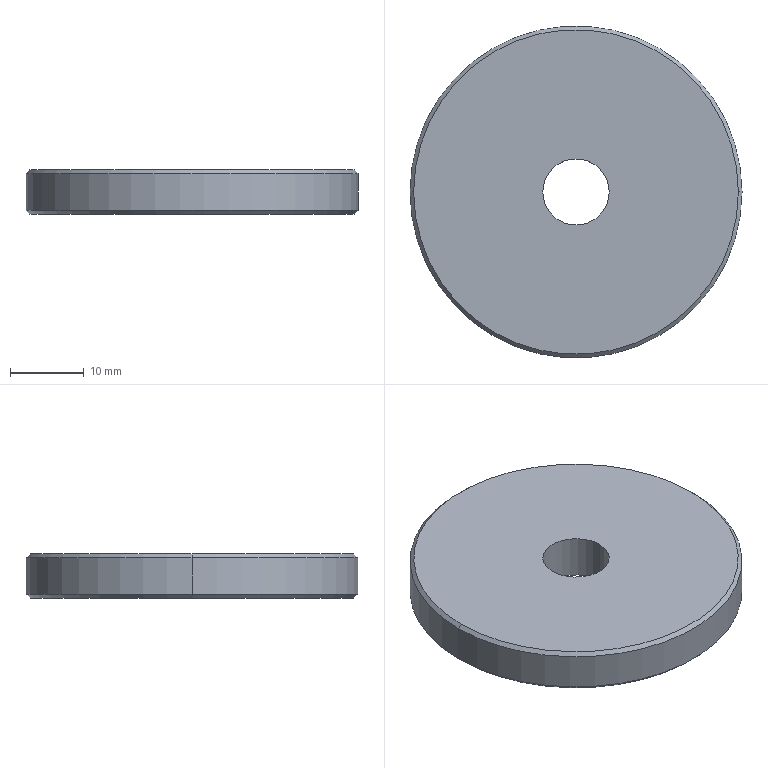Part | SolidWorks | features Chamfer 1, Extrusion 1 | 1 solid | 10 faces | box 45 x 45 x 6 mm | volume 9126 mm3 | cone 4 | cylinder 4 | plane 2 | commonest cylinder face diameters 9 x2 45 x2
STEP:
#1=CARTESIAN_POINT('',(22.,0.,6.));
#2=VERTEX_POINT('',#1);
#3=CARTESIAN_POINT('',(-22.,0.,6.));
#4=VERTEX_POINT('',#3);
#5=CARTESIAN_POINT('',(0.,0.,6.));
#6=DIRECTION('',(0.,0.,1.));
#7=DIRECTION('',(1.,0.,0.));
#8=AXIS2_PLACEMENT_3D('',#5,#6,#7);
#9=CIRCLE('',#8,22.);
#10=EDGE_CURVE('',#2,#4,#9,.T.);
#11=ORIENTED_EDGE('',*,*,#10,.F.);
#12=CARTESIAN_POINT('',(22.5,0.,5.5));
#13=VERTEX_POINT('',#12);
#14=CARTESIAN_POINT('',(22.,0.,6.));
#15=DIRECTION('',(0.7071,0.,-0.7071));
#16=VECTOR('',#15,1000.);
#17=LINE('',#14,#16);
#18=EDGE_CURVE('',#2,#13,#17,.T.);
#19=ORIENTED_EDGE('',*,*,#18,.T.);
#20=CARTESIAN_POINT('',(-22.5,0.,5.5));
#21=VERTEX_POINT('',#20);
#22=CARTESIAN_POINT('',(0.,0.,5.5));
#23=DIRECTION('',(0.,0.,-1.));
#24=DIRECTION('',(1.,0.,0.));
#25=AXIS2_PLACEMENT_3D('',#22,#23,#24);
#26=CIRCLE('',#25,22.5);
#27=EDGE_CURVE('',#21,#13,#26,.T.);
#28=ORIENTED_EDGE('',*,*,#27,.F.);
#29=CARTESIAN_POINT('',(-22.,0.,6.));
#30=DIRECTION('',(-0.7071,0.,-0.7071));
#31=VECTOR('',#30,1000.);
#32=LINE('',#29,#31);
#33=EDGE_CURVE('',#4,#21,#32,.T.);
#34=ORIENTED_EDGE('',*,*,#33,.F.);
#35=EDGE_LOOP('',(#11,#19,#28,#34));
#36=FACE_OUTER_BOUND('',#35,.T.);
#37=CARTESIAN_POINT('',(0.,0.,6.));
#38=DIRECTION('',(0.,0.,-1.));
#39=DIRECTION('',(-1.,0.,0.));
#40=AXIS2_PLACEMENT_3D('',#37,#38,#39);
#41=CONICAL_SURFACE('',#40,22.,0.7854);
#42=ADVANCED_FACE('',(#36),#41,.T.);
#43=CARTESIAN_POINT('',(-22.,0.,0.));
#44=VERTEX_POINT('',#43);
#45=CARTESIAN_POINT('',(22.,0.,0.));
#46=VERTEX_POINT('',#45);
#47=CARTESIAN_POINT('',(0.,0.,0.));
#48=DIRECTION('',(0.,0.,-1.));
#49=DIRECTION('',(1.,0.,0.));
#50=AXIS2_PLACEMENT_3D('',#47,#48,#49);
#51=CIRCLE('',#50,22.);
#52=EDGE_CURVE('',#44,#46,#51,.T.);
#53=ORIENTED_EDGE('',*,*,#52,.F.);
#54=CARTESIAN_POINT('',(-22.5,0.,0.5));
#55=VERTEX_POINT('',#54);
#56=CARTESIAN_POINT('',(-22.5,0.,0.5));
#57=DIRECTION('',(-0.7071,0.,0.7071));
#58=VECTOR('',#57,1000.);
#59=LINE('',#56,#58);
#60=EDGE_CURVE('',#44,#55,#59,.T.);
#61=ORIENTED_EDGE('',*,*,#60,.T.);
#62=CARTESIAN_POINT('',(22.5,0.,0.5));
#63=VERTEX_POINT('',#62);
#64=CARTESIAN_POINT('',(0.,0.,0.5));
#65=DIRECTION('',(0.,0.,1.));
#66=DIRECTION('',(1.,0.,0.));
#67=AXIS2_PLACEMENT_3D('',#64,#65,#66);
#68=CIRCLE('',#67,22.5);
#69=EDGE_CURVE('',#63,#55,#68,.T.);
#70=ORIENTED_EDGE('',*,*,#69,.F.);
#71=CARTESIAN_POINT('',(22.5,0.,0.5));
#72=DIRECTION('',(0.7071,0.,0.7071));
#73=VECTOR('',#72,1000.);
#74=LINE('',#71,#73);
#75=EDGE_CURVE('',#46,#63,#74,.T.);
#76=ORIENTED_EDGE('',*,*,#75,.F.);
#77=EDGE_LOOP('',(#53,#61,#70,#76));
#78=FACE_OUTER_BOUND('',#77,.T.);
#79=CARTESIAN_POINT('',(0.,0.,0.5));
#80=DIRECTION('',(0.,0.,1.));
#81=DIRECTION('',(1.,0.,0.));
#82=AXIS2_PLACEMENT_3D('',#79,#80,#81);
#83=CONICAL_SURFACE('',#82,22.5,0.7854);
#84=ADVANCED_FACE('',(#78),#83,.T.);
#85=CARTESIAN_POINT('',(-4.5,0.,6.));
#86=VERTEX_POINT('',#85);
#87=CARTESIAN_POINT('',(4.5,0.,6.));
#88=VERTEX_POINT('',#87);
#89=CARTESIAN_POINT('',(0.,0.,6.));
#90=DIRECTION('',(0.,0.,1.));
#91=DIRECTION('',(1.,0.,0.));
#92=AXIS2_PLACEMENT_3D('',#89,#90,#91);
#93=CIRCLE('',#92,4.5);
#94=EDGE_CURVE('',#86,#88,#93,.T.);
#95=ORIENTED_EDGE('',*,*,#94,.T.);
#96=CARTESIAN_POINT('',(4.5,0.,0.));
#97=VERTEX_POINT('',#96);
#98=CARTESIAN_POINT('',(4.5,0.,6.));
#99=DIRECTION('',(0.,0.,-1.));
#100=VECTOR('',#99,1000.);
#101=LINE('',#98,#100);
#102=EDGE_CURVE('',#88,#97,#101,.T.);
#103=ORIENTED_EDGE('',*,*,#102,.T.);
#104=CARTESIAN_POINT('',(-4.5,0.,0.));
#105=VERTEX_POINT('',#104);
#106=CARTESIAN_POINT('',(0.,0.,0.));
#107=DIRECTION('',(0.,0.,1.));
#108=DIRECTION('',(1.,0.,0.));
#109=AXIS2_PLACEMENT_3D('',#106,#107,#108);
#110=CIRCLE('',#109,4.5);
#111=EDGE_CURVE('',#105,#97,#110,.T.);
#112=ORIENTED_EDGE('',*,*,#111,.F.);
#113=CARTESIAN_POINT('',(-4.5,0.,6.));
#114=DIRECTION('',(0.,0.,-1.));
#115=VECTOR('',#114,1000.);
#116=LINE('',#113,#115);
#117=EDGE_CURVE('',#86,#105,#116,.T.);
#118=ORIENTED_EDGE('',*,*,#117,.F.);
#119=EDGE_LOOP('',(#95,#103,#112,#118));
#120=FACE_OUTER_BOUND('',#119,.T.);
#121=CARTESIAN_POINT('',(0.,0.,6.));
#122=DIRECTION('',(0.,0.,-1.));
#123=DIRECTION('',(-1.,0.,0.));
#124=AXIS2_PLACEMENT_3D('',#121,#122,#123);
#125=CYLINDRICAL_SURFACE('',#124,4.5);
#126=ADVANCED_FACE('',(#120),#125,.F.);
#127=ORIENTED_EDGE('',*,*,#27,.T.);
#128=CARTESIAN_POINT('',(22.5,0.,6.));
#129=DIRECTION('',(0.,0.,-1.));
#130=VECTOR('',#129,1000.);
#131=LINE('',#128,#130);
#132=EDGE_CURVE('',#13,#63,#131,.T.);
#133=ORIENTED_EDGE('',*,*,#132,.T.);
#134=ORIENTED_EDGE('',*,*,#69,.T.);
#135=CARTESIAN_POINT('',(-22.5,0.,6.));
#136=DIRECTION('',(0.,0.,-1.));
#137=VECTOR('',#136,1000.);
#138=LINE('',#135,#137);
#139=EDGE_CURVE('',#21,#55,#138,.T.);
#140=ORIENTED_EDGE('',*,*,#139,.F.);
#141=EDGE_LOOP('',(#127,#133,#134,#140));
#142=FACE_OUTER_BOUND('',#141,.T.);
#143=CARTESIAN_POINT('',(0.,0.,6.));
#144=DIRECTION('',(0.,0.,-1.));
#145=DIRECTION('',(-1.,0.,0.));
#146=AXIS2_PLACEMENT_3D('',#143,#144,#145);
#147=CYLINDRICAL_SURFACE('',#146,22.5);
#148=ADVANCED_FACE('',(#142),#147,.T.);
#149=CARTESIAN_POINT('',(0.,0.,6.));
#150=DIRECTION('',(0.,0.,1.));
#151=DIRECTION('',(1.,0.,0.));
#152=AXIS2_PLACEMENT_3D('',#149,#150,#151);
#153=CIRCLE('',#152,22.);
#154=EDGE_CURVE('',#4,#2,#153,.T.);
#155=ORIENTED_EDGE('',*,*,#154,.T.);
#156=ORIENTED_EDGE('',*,*,#10,.T.);
#157=EDGE_LOOP('',(#155,#156));
#158=FACE_OUTER_BOUND('',#157,.T.);
#159=ORIENTED_EDGE('',*,*,#94,.F.);
#160=CARTESIAN_POINT('',(0.,0.,6.));
#161=DIRECTION('',(0.,0.,1.));
#162=DIRECTION('',(1.,0.,0.));
#163=AXIS2_PLACEMENT_3D('',#160,#161,#162);
#164=CIRCLE('',#163,4.5);
#165=EDGE_CURVE('',#88,#86,#164,.T.);
#166=ORIENTED_EDGE('',*,*,#165,.F.);
#167=EDGE_LOOP('',(#159,#166));
#168=FACE_BOUND('',#167,.T.);
#169=CARTESIAN_POINT('',(0.,0.,6.));
#170=DIRECTION('',(0.,0.,1.));
#171=DIRECTION('',(1.,0.,0.));
#172=AXIS2_PLACEMENT_3D('',#169,#170,#171);
#173=PLANE('',#172);
#174=ADVANCED_FACE('',(#158,#168),#173,.T.);
#175=CARTESIAN_POINT('',(0.,0.,0.));
#176=DIRECTION('',(0.,0.,-1.));
#177=DIRECTION('',(1.,0.,0.));
#178=AXIS2_PLACEMENT_3D('',#175,#176,#177);
#179=CIRCLE('',#178,22.);
#180=EDGE_CURVE('',#46,#44,#179,.T.);
#181=ORIENTED_EDGE('',*,*,#180,.T.);
#182=ORIENTED_EDGE('',*,*,#52,.T.);
#183=EDGE_LOOP('',(#181,#182));
#184=FACE_OUTER_BOUND('',#183,.T.);
#185=ORIENTED_EDGE('',*,*,#111,.T.);
#186=CARTESIAN_POINT('',(0.,0.,0.));
#187=DIRECTION('',(0.,0.,1.));
#188=DIRECTION('',(1.,0.,0.));
#189=AXIS2_PLACEMENT_3D('',#186,#187,#188);
#190=CIRCLE('',#189,4.5);
#191=EDGE_CURVE('',#97,#105,#190,.T.);
#192=ORIENTED_EDGE('',*,*,#191,.T.);
#193=EDGE_LOOP('',(#185,#192));
#194=FACE_BOUND('',#193,.T.);
#195=CARTESIAN_POINT('',(0.,0.,0.));
#196=DIRECTION('',(0.,0.,1.));
#197=DIRECTION('',(1.,0.,0.));
#198=AXIS2_PLACEMENT_3D('',#195,#196,#197);
#199=PLANE('',#198);
#200=ADVANCED_FACE('',(#184,#194),#199,.F.);
#201=ORIENTED_EDGE('',*,*,#132,.F.);
#202=CARTESIAN_POINT('',(0.,0.,5.5));
#203=DIRECTION('',(0.,0.,-1.));
#204=DIRECTION('',(1.,0.,0.));
#205=AXIS2_PLACEMENT_3D('',#202,#203,#204);
#206=CIRCLE('',#205,22.5);
#207=EDGE_CURVE('',#13,#21,#206,.T.);
#208=ORIENTED_EDGE('',*,*,#207,.T.);
#209=ORIENTED_EDGE('',*,*,#139,.T.);
#210=CARTESIAN_POINT('',(0.,0.,0.5));
#211=DIRECTION('',(0.,0.,1.));
#212=DIRECTION('',(1.,0.,0.));
#213=AXIS2_PLACEMENT_3D('',#210,#211,#212);
#214=CIRCLE('',#213,22.5);
#215=EDGE_CURVE('',#55,#63,#214,.T.);
#216=ORIENTED_EDGE('',*,*,#215,.T.);
#217=EDGE_LOOP('',(#201,#208,#209,#216));
#218=FACE_OUTER_BOUND('',#217,.T.);
#219=CARTESIAN_POINT('',(0.,0.,6.));
#220=DIRECTION('',(0.,0.,-1.));
#221=DIRECTION('',(-1.,0.,0.));
#222=AXIS2_PLACEMENT_3D('',#219,#220,#221);
#223=CYLINDRICAL_SURFACE('',#222,22.5);
#224=ADVANCED_FACE('',(#218),#223,.T.);
#225=ORIENTED_EDGE('',*,*,#102,.F.);
#226=ORIENTED_EDGE('',*,*,#165,.T.);
#227=ORIENTED_EDGE('',*,*,#117,.T.);
#228=ORIENTED_EDGE('',*,*,#191,.F.);
#229=EDGE_LOOP('',(#225,#226,#227,#228));
#230=FACE_OUTER_BOUND('',#229,.T.);
#231=CARTESIAN_POINT('',(0.,0.,6.));
#232=DIRECTION('',(0.,0.,-1.));
#233=DIRECTION('',(-1.,0.,0.));
#234=AXIS2_PLACEMENT_3D('',#231,#232,#233);
#235=CYLINDRICAL_SURFACE('',#234,4.5);
#236=ADVANCED_FACE('',(#230),#235,.F.);
#237=ORIENTED_EDGE('',*,*,#60,.F.);
#238=ORIENTED_EDGE('',*,*,#180,.F.);
#239=ORIENTED_EDGE('',*,*,#75,.T.);
#240=ORIENTED_EDGE('',*,*,#215,.F.);
#241=EDGE_LOOP('',(#237,#238,#239,#240));
#242=FACE_OUTER_BOUND('',#241,.T.);
#243=CARTESIAN_POINT('',(0.,0.,0.5));
#244=DIRECTION('',(0.,0.,1.));
#245=DIRECTION('',(1.,0.,0.));
#246=AXIS2_PLACEMENT_3D('',#243,#244,#245);
#247=CONICAL_SURFACE('',#246,22.5,0.7854);
#248=ADVANCED_FACE('',(#242),#247,.T.);
#249=ORIENTED_EDGE('',*,*,#18,.F.);
#250=ORIENTED_EDGE('',*,*,#154,.F.);
#251=ORIENTED_EDGE('',*,*,#33,.T.);
#252=ORIENTED_EDGE('',*,*,#207,.F.);
#253=EDGE_LOOP('',(#249,#250,#251,#252));
#254=FACE_OUTER_BOUND('',#253,.T.);
#255=CARTESIAN_POINT('',(0.,0.,6.));
#256=DIRECTION('',(0.,0.,-1.));
#257=DIRECTION('',(-1.,0.,0.));
#258=AXIS2_PLACEMENT_3D('',#255,#256,#257);
#259=CONICAL_SURFACE('',#258,22.,0.7854);
#260=ADVANCED_FACE('',(#254),#259,.T.);
#261=CLOSED_SHELL('',(#42,#84,#126,#148,#174,#200,#224,#236,#248,#260));
#262=MANIFOLD_SOLID_BREP('',#261);
#263=CARTESIAN_POINT('',(0.,0.,0.));
#264=DIRECTION('',(0.,0.,1.));
#265=DIRECTION('',(1.,0.,0.));
#266=AXIS2_PLACEMENT_3D('',#263,#264,#265);
#267=(LENGTH_UNIT()NAMED_UNIT(*)SI_UNIT(.MILLI.,.METRE.));
#268=UNCERTAINTY_MEASURE_WITH_UNIT(LENGTH_MEASURE(0.00001),#267,'','');
#269=(NAMED_UNIT(*)PLANE_ANGLE_UNIT()SI_UNIT($,.RADIAN.));
#270=(NAMED_UNIT(*)SI_UNIT($,.STERADIAN.)SOLID_ANGLE_UNIT());
#271=(GEOMETRIC_REPRESENTATION_CONTEXT(3)GLOBAL_UNCERTAINTY_ASSIGNED_CONTEXT((#268))GLOBAL_UNIT_ASSIGNED_CONTEXT((#267,#269,#270))REPRESENTATION_CONTEXT('',''));
#272=ADVANCED_BREP_SHAPE_REPRESENTATION('',(#262,#266),#271);